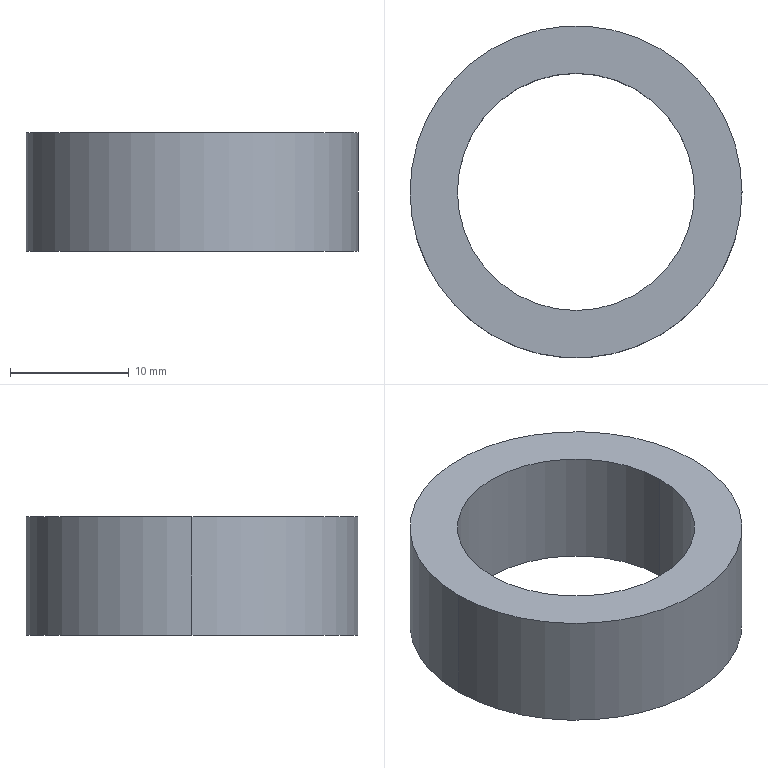Part | SolidWorks | features Extrusion 1 | 1 solid | 6 faces | box 28 x 28 x 10 mm | volume 3016 mm3 | cylinder 4 | plane 2 | commonest cylinder face diameters 20 x2 28 x2
STEP:
#1=CARTESIAN_POINT('',(-10.,0.,10.));
#2=VERTEX_POINT('',#1);
#3=CARTESIAN_POINT('',(10.,0.,10.));
#4=VERTEX_POINT('',#3);
#5=CARTESIAN_POINT('',(0.,0.,10.));
#6=DIRECTION('',(0.,0.,1.));
#7=DIRECTION('',(1.,0.,0.));
#8=AXIS2_PLACEMENT_3D('',#5,#6,#7);
#9=CIRCLE('',#8,10.);
#10=EDGE_CURVE('',#2,#4,#9,.T.);
#11=ORIENTED_EDGE('',*,*,#10,.T.);
#12=CARTESIAN_POINT('',(10.,0.,0.));
#13=VERTEX_POINT('',#12);
#14=CARTESIAN_POINT('',(10.,0.,10.));
#15=DIRECTION('',(0.,0.,-1.));
#16=VECTOR('',#15,1000.);
#17=LINE('',#14,#16);
#18=EDGE_CURVE('',#4,#13,#17,.T.);
#19=ORIENTED_EDGE('',*,*,#18,.T.);
#20=CARTESIAN_POINT('',(-10.,0.,0.));
#21=VERTEX_POINT('',#20);
#22=CARTESIAN_POINT('',(0.,0.,0.));
#23=DIRECTION('',(0.,0.,1.));
#24=DIRECTION('',(1.,0.,0.));
#25=AXIS2_PLACEMENT_3D('',#22,#23,#24);
#26=CIRCLE('',#25,10.);
#27=EDGE_CURVE('',#21,#13,#26,.T.);
#28=ORIENTED_EDGE('',*,*,#27,.F.);
#29=CARTESIAN_POINT('',(-10.,0.,10.));
#30=DIRECTION('',(0.,0.,-1.));
#31=VECTOR('',#30,1000.);
#32=LINE('',#29,#31);
#33=EDGE_CURVE('',#2,#21,#32,.T.);
#34=ORIENTED_EDGE('',*,*,#33,.F.);
#35=EDGE_LOOP('',(#11,#19,#28,#34));
#36=FACE_OUTER_BOUND('',#35,.T.);
#37=CARTESIAN_POINT('',(0.,0.,10.));
#38=DIRECTION('',(0.,0.,-1.));
#39=DIRECTION('',(-1.,0.,0.));
#40=AXIS2_PLACEMENT_3D('',#37,#38,#39);
#41=CYLINDRICAL_SURFACE('',#40,10.);
#42=ADVANCED_FACE('',(#36),#41,.F.);
#43=CARTESIAN_POINT('',(14.,0.,10.));
#44=VERTEX_POINT('',#43);
#45=CARTESIAN_POINT('',(-14.,0.,10.));
#46=VERTEX_POINT('',#45);
#47=CARTESIAN_POINT('',(0.,0.,10.));
#48=DIRECTION('',(0.,0.,1.));
#49=DIRECTION('',(1.,0.,0.));
#50=AXIS2_PLACEMENT_3D('',#47,#48,#49);
#51=CIRCLE('',#50,14.);
#52=EDGE_CURVE('',#44,#46,#51,.T.);
#53=ORIENTED_EDGE('',*,*,#52,.F.);
#54=CARTESIAN_POINT('',(14.,0.,0.));
#55=VERTEX_POINT('',#54);
#56=CARTESIAN_POINT('',(14.,0.,10.));
#57=DIRECTION('',(0.,0.,-1.));
#58=VECTOR('',#57,1000.);
#59=LINE('',#56,#58);
#60=EDGE_CURVE('',#44,#55,#59,.T.);
#61=ORIENTED_EDGE('',*,*,#60,.T.);
#62=CARTESIAN_POINT('',(-14.,0.,0.));
#63=VERTEX_POINT('',#62);
#64=CARTESIAN_POINT('',(0.,0.,0.));
#65=DIRECTION('',(0.,0.,1.));
#66=DIRECTION('',(1.,0.,0.));
#67=AXIS2_PLACEMENT_3D('',#64,#65,#66);
#68=CIRCLE('',#67,14.);
#69=EDGE_CURVE('',#55,#63,#68,.T.);
#70=ORIENTED_EDGE('',*,*,#69,.T.);
#71=CARTESIAN_POINT('',(-14.,0.,10.));
#72=DIRECTION('',(0.,0.,-1.));
#73=VECTOR('',#72,1000.);
#74=LINE('',#71,#73);
#75=EDGE_CURVE('',#46,#63,#74,.T.);
#76=ORIENTED_EDGE('',*,*,#75,.F.);
#77=EDGE_LOOP('',(#53,#61,#70,#76));
#78=FACE_OUTER_BOUND('',#77,.T.);
#79=CARTESIAN_POINT('',(0.,0.,10.));
#80=DIRECTION('',(0.,0.,-1.));
#81=DIRECTION('',(-1.,0.,0.));
#82=AXIS2_PLACEMENT_3D('',#79,#80,#81);
#83=CYLINDRICAL_SURFACE('',#82,14.);
#84=ADVANCED_FACE('',(#78),#83,.T.);
#85=CARTESIAN_POINT('',(0.,0.,10.));
#86=DIRECTION('',(0.,0.,1.));
#87=DIRECTION('',(1.,0.,0.));
#88=AXIS2_PLACEMENT_3D('',#85,#86,#87);
#89=CIRCLE('',#88,14.);
#90=EDGE_CURVE('',#46,#44,#89,.T.);
#91=ORIENTED_EDGE('',*,*,#90,.T.);
#92=ORIENTED_EDGE('',*,*,#52,.T.);
#93=EDGE_LOOP('',(#91,#92));
#94=FACE_OUTER_BOUND('',#93,.T.);
#95=ORIENTED_EDGE('',*,*,#10,.F.);
#96=CARTESIAN_POINT('',(0.,0.,10.));
#97=DIRECTION('',(0.,0.,1.));
#98=DIRECTION('',(1.,0.,0.));
#99=AXIS2_PLACEMENT_3D('',#96,#97,#98);
#100=CIRCLE('',#99,10.);
#101=EDGE_CURVE('',#4,#2,#100,.T.);
#102=ORIENTED_EDGE('',*,*,#101,.F.);
#103=EDGE_LOOP('',(#95,#102));
#104=FACE_BOUND('',#103,.T.);
#105=CARTESIAN_POINT('',(0.,0.,10.));
#106=DIRECTION('',(0.,0.,1.));
#107=DIRECTION('',(1.,0.,0.));
#108=AXIS2_PLACEMENT_3D('',#105,#106,#107);
#109=PLANE('',#108);
#110=ADVANCED_FACE('',(#94,#104),#109,.T.);
#111=CARTESIAN_POINT('',(0.,0.,0.));
#112=DIRECTION('',(0.,0.,1.));
#113=DIRECTION('',(1.,0.,0.));
#114=AXIS2_PLACEMENT_3D('',#111,#112,#113);
#115=CIRCLE('',#114,14.);
#116=EDGE_CURVE('',#63,#55,#115,.T.);
#117=ORIENTED_EDGE('',*,*,#116,.F.);
#118=ORIENTED_EDGE('',*,*,#69,.F.);
#119=EDGE_LOOP('',(#117,#118));
#120=FACE_OUTER_BOUND('',#119,.T.);
#121=ORIENTED_EDGE('',*,*,#27,.T.);
#122=CARTESIAN_POINT('',(0.,0.,0.));
#123=DIRECTION('',(0.,0.,1.));
#124=DIRECTION('',(1.,0.,0.));
#125=AXIS2_PLACEMENT_3D('',#122,#123,#124);
#126=CIRCLE('',#125,10.);
#127=EDGE_CURVE('',#13,#21,#126,.T.);
#128=ORIENTED_EDGE('',*,*,#127,.T.);
#129=EDGE_LOOP('',(#121,#128));
#130=FACE_BOUND('',#129,.T.);
#131=CARTESIAN_POINT('',(0.,0.,0.));
#132=DIRECTION('',(0.,0.,1.));
#133=DIRECTION('',(1.,0.,0.));
#134=AXIS2_PLACEMENT_3D('',#131,#132,#133);
#135=PLANE('',#134);
#136=ADVANCED_FACE('',(#120,#130),#135,.F.);
#137=ORIENTED_EDGE('',*,*,#60,.F.);
#138=ORIENTED_EDGE('',*,*,#90,.F.);
#139=ORIENTED_EDGE('',*,*,#75,.T.);
#140=ORIENTED_EDGE('',*,*,#116,.T.);
#141=EDGE_LOOP('',(#137,#138,#139,#140));
#142=FACE_OUTER_BOUND('',#141,.T.);
#143=CARTESIAN_POINT('',(0.,0.,10.));
#144=DIRECTION('',(0.,0.,-1.));
#145=DIRECTION('',(-1.,0.,0.));
#146=AXIS2_PLACEMENT_3D('',#143,#144,#145);
#147=CYLINDRICAL_SURFACE('',#146,14.);
#148=ADVANCED_FACE('',(#142),#147,.T.);
#149=ORIENTED_EDGE('',*,*,#18,.F.);
#150=ORIENTED_EDGE('',*,*,#101,.T.);
#151=ORIENTED_EDGE('',*,*,#33,.T.);
#152=ORIENTED_EDGE('',*,*,#127,.F.);
#153=EDGE_LOOP('',(#149,#150,#151,#152));
#154=FACE_OUTER_BOUND('',#153,.T.);
#155=CARTESIAN_POINT('',(0.,0.,10.));
#156=DIRECTION('',(0.,0.,-1.));
#157=DIRECTION('',(-1.,0.,0.));
#158=AXIS2_PLACEMENT_3D('',#155,#156,#157);
#159=CYLINDRICAL_SURFACE('',#158,10.);
#160=ADVANCED_FACE('',(#154),#159,.F.);
#161=CLOSED_SHELL('',(#42,#84,#110,#136,#148,#160));
#162=MANIFOLD_SOLID_BREP('',#161);
#163=CARTESIAN_POINT('',(0.,0.,0.));
#164=DIRECTION('',(0.,0.,1.));
#165=DIRECTION('',(1.,0.,0.));
#166=AXIS2_PLACEMENT_3D('',#163,#164,#165);
#167=(LENGTH_UNIT()NAMED_UNIT(*)SI_UNIT(.MILLI.,.METRE.));
#168=UNCERTAINTY_MEASURE_WITH_UNIT(LENGTH_MEASURE(0.00001),#167,'','');
#169=(NAMED_UNIT(*)PLANE_ANGLE_UNIT()SI_UNIT($,.RADIAN.));
#170=(NAMED_UNIT(*)SI_UNIT($,.STERADIAN.)SOLID_ANGLE_UNIT());
#171=(GEOMETRIC_REPRESENTATION_CONTEXT(3)GLOBAL_UNCERTAINTY_ASSIGNED_CONTEXT((#168))GLOBAL_UNIT_ASSIGNED_CONTEXT((#167,#169,#170))REPRESENTATION_CONTEXT('',''));
#172=ADVANCED_BREP_SHAPE_REPRESENTATION('',(#162,#166),#171);